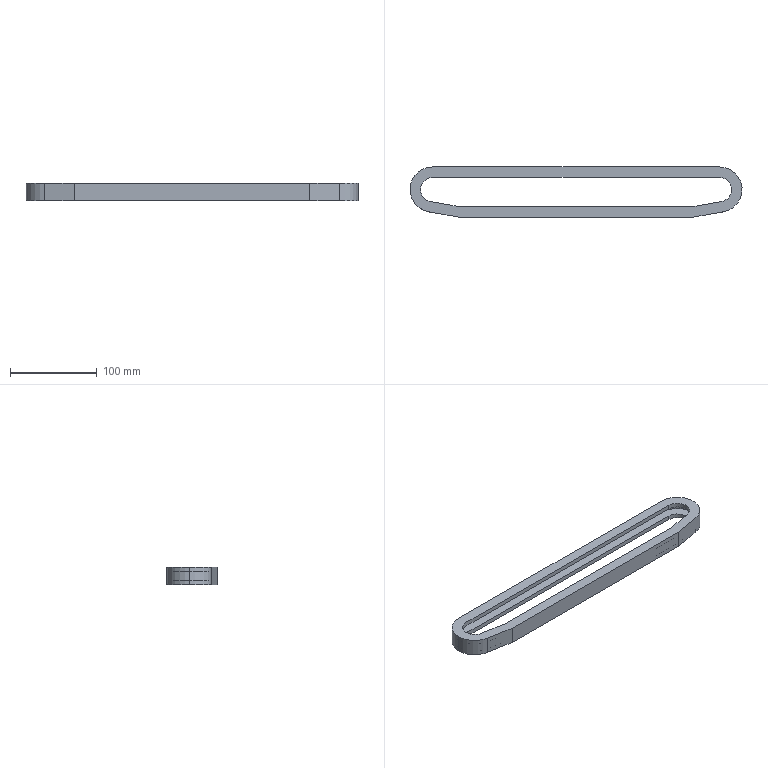Part | SolidWorks | features Extrusion 1, ICE 1 | 1 solid | 32 faces | box 382 x 57.598 x 20 mm | volume 102612 mm3 | plane 20 | cylinder 12 | commonest cylinder face diameters 28 x6 50 x3 52 x3
STEP:
#1=CARTESIAN_POINT('',(190.,0.,-5.));
#2=VERTEX_POINT('',#1);
#3=CARTESIAN_POINT('',(165.,25.,-5.));
#4=VERTEX_POINT('',#3);
#5=CARTESIAN_POINT('',(165.,0.,-5.));
#6=DIRECTION('',(0.,0.,1.));
#7=DIRECTION('',(1.,0.,0.));
#8=AXIS2_PLACEMENT_3D('',#5,#6,#7);
#9=CIRCLE('',#8,25.);
#10=EDGE_CURVE('',#2,#4,#9,.T.);
#11=ORIENTED_EDGE('',*,*,#10,.F.);
#12=CARTESIAN_POINT('',(190.,0.,5.));
#13=VERTEX_POINT('',#12);
#14=CARTESIAN_POINT('',(190.,0.,-5.));
#15=DIRECTION('',(0.,0.,1.));
#16=VECTOR('',#15,1000.);
#17=LINE('',#14,#16);
#18=EDGE_CURVE('',#2,#13,#17,.T.);
#19=ORIENTED_EDGE('',*,*,#18,.T.);
#20=CARTESIAN_POINT('',(165.,25.,5.));
#21=VERTEX_POINT('',#20);
#22=CARTESIAN_POINT('',(165.,0.,5.));
#23=DIRECTION('',(0.,0.,1.));
#24=DIRECTION('',(1.,0.,0.));
#25=AXIS2_PLACEMENT_3D('',#22,#23,#24);
#26=CIRCLE('',#25,25.);
#27=EDGE_CURVE('',#13,#21,#26,.T.);
#28=ORIENTED_EDGE('',*,*,#27,.T.);
#29=CARTESIAN_POINT('',(165.,25.,-5.));
#30=DIRECTION('',(0.,0.,1.));
#31=VECTOR('',#30,1000.);
#32=LINE('',#29,#31);
#33=EDGE_CURVE('',#4,#21,#32,.T.);
#34=ORIENTED_EDGE('',*,*,#33,.F.);
#35=EDGE_LOOP('',(#11,#19,#28,#34));
#36=FACE_OUTER_BOUND('',#35,.T.);
#37=CARTESIAN_POINT('',(165.,0.,-5.));
#38=DIRECTION('',(0.,0.,1.));
#39=DIRECTION('',(1.,0.,0.));
#40=AXIS2_PLACEMENT_3D('',#37,#38,#39);
#41=CYLINDRICAL_SURFACE('',#40,25.);
#42=ADVANCED_FACE('',(#36),#41,.F.);
#43=CARTESIAN_POINT('',(-165.,14.,10.));
#44=VERTEX_POINT('',#43);
#45=CARTESIAN_POINT('',(-179.,0.,10.));
#46=VERTEX_POINT('',#45);
#47=CARTESIAN_POINT('',(-165.,0.,10.));
#48=DIRECTION('',(0.,0.,1.));
#49=DIRECTION('',(1.,0.,0.));
#50=AXIS2_PLACEMENT_3D('',#47,#48,#49);
#51=CIRCLE('',#50,14.);
#52=EDGE_CURVE('',#44,#46,#51,.T.);
#53=ORIENTED_EDGE('',*,*,#52,.T.);
#54=CARTESIAN_POINT('',(-179.,0.,5.));
#55=VERTEX_POINT('',#54);
#56=CARTESIAN_POINT('',(-179.,0.,10.));
#57=DIRECTION('',(0.,0.,-1.));
#58=VECTOR('',#57,1000.);
#59=LINE('',#56,#58);
#60=EDGE_CURVE('',#46,#55,#59,.T.);
#61=ORIENTED_EDGE('',*,*,#60,.T.);
#62=CARTESIAN_POINT('',(-165.,14.,5.));
#63=VERTEX_POINT('',#62);
#64=CARTESIAN_POINT('',(-165.,0.,5.));
#65=DIRECTION('',(0.,0.,1.));
#66=DIRECTION('',(1.,0.,0.));
#67=AXIS2_PLACEMENT_3D('',#64,#65,#66);
#68=CIRCLE('',#67,14.);
#69=EDGE_CURVE('',#63,#55,#68,.T.);
#70=ORIENTED_EDGE('',*,*,#69,.F.);
#71=CARTESIAN_POINT('',(-165.,14.,10.));
#72=DIRECTION('',(0.,0.,-1.));
#73=VECTOR('',#72,1000.);
#74=LINE('',#71,#73);
#75=EDGE_CURVE('',#44,#63,#74,.T.);
#76=ORIENTED_EDGE('',*,*,#75,.F.);
#77=EDGE_LOOP('',(#53,#61,#70,#76));
#78=FACE_OUTER_BOUND('',#77,.T.);
#79=CARTESIAN_POINT('',(-165.,0.,10.));
#80=DIRECTION('',(0.,0.,-1.));
#81=DIRECTION('',(-1.,0.,0.));
#82=AXIS2_PLACEMENT_3D('',#79,#80,#81);
#83=CYLINDRICAL_SURFACE('',#82,14.);
#84=ADVANCED_FACE('',(#78),#83,.F.);
#85=CARTESIAN_POINT('',(-191.,0.,10.));
#86=VERTEX_POINT('',#85);
#87=CARTESIAN_POINT('',(-169.515,-25.605,10.));
#88=VERTEX_POINT('',#87);
#89=CARTESIAN_POINT('',(-165.,0.,10.));
#90=DIRECTION('',(0.,0.,1.));
#91=DIRECTION('',(1.,0.,0.));
#92=AXIS2_PLACEMENT_3D('',#89,#90,#91);
#93=CIRCLE('',#92,26.);
#94=EDGE_CURVE('',#86,#88,#93,.T.);
#95=ORIENTED_EDGE('',*,*,#94,.F.);
#96=CARTESIAN_POINT('',(-191.,0.,-10.));
#97=VERTEX_POINT('',#96);
#98=CARTESIAN_POINT('',(-191.,0.,10.));
#99=DIRECTION('',(0.,0.,-1.));
#100=VECTOR('',#99,1000.);
#101=LINE('',#98,#100);
#102=EDGE_CURVE('',#86,#97,#101,.T.);
#103=ORIENTED_EDGE('',*,*,#102,.T.);
#104=CARTESIAN_POINT('',(-169.515,-25.605,-10.));
#105=VERTEX_POINT('',#104);
#106=CARTESIAN_POINT('',(-165.,0.,-10.));
#107=DIRECTION('',(0.,0.,1.));
#108=DIRECTION('',(1.,0.,0.));
#109=AXIS2_PLACEMENT_3D('',#106,#107,#108);
#110=CIRCLE('',#109,26.);
#111=EDGE_CURVE('',#97,#105,#110,.T.);
#112=ORIENTED_EDGE('',*,*,#111,.T.);
#113=CARTESIAN_POINT('',(-169.515,-25.605,10.));
#114=DIRECTION('',(0.,0.,-1.));
#115=VECTOR('',#114,1000.);
#116=LINE('',#113,#115);
#117=EDGE_CURVE('',#88,#105,#116,.T.);
#118=ORIENTED_EDGE('',*,*,#117,.F.);
#119=EDGE_LOOP('',(#95,#103,#112,#118));
#120=FACE_OUTER_BOUND('',#119,.T.);
#121=CARTESIAN_POINT('',(-165.,0.,10.));
#122=DIRECTION('',(0.,0.,-1.));
#123=DIRECTION('',(-1.,0.,0.));
#124=AXIS2_PLACEMENT_3D('',#121,#122,#123);
#125=CYLINDRICAL_SURFACE('',#124,26.);
#126=ADVANCED_FACE('',(#120),#125,.T.);
#127=CARTESIAN_POINT('',(-165.,14.,-5.));
#128=VERTEX_POINT('',#127);
#129=CARTESIAN_POINT('',(-179.,0.,-5.));
#130=VERTEX_POINT('',#129);
#131=CARTESIAN_POINT('',(-165.,0.,-5.));
#132=DIRECTION('',(0.,0.,1.));
#133=DIRECTION('',(1.,0.,0.));
#134=AXIS2_PLACEMENT_3D('',#131,#132,#133);
#135=CIRCLE('',#134,14.);
#136=EDGE_CURVE('',#128,#130,#135,.T.);
#137=ORIENTED_EDGE('',*,*,#136,.T.);
#138=CARTESIAN_POINT('',(-179.,0.,-10.));
#139=VERTEX_POINT('',#138);
#140=CARTESIAN_POINT('',(-179.,0.,10.));
#141=DIRECTION('',(0.,0.,-1.));
#142=VECTOR('',#141,1000.);
#143=LINE('',#140,#142);
#144=EDGE_CURVE('',#130,#139,#143,.T.);
#145=ORIENTED_EDGE('',*,*,#144,.T.);
#146=CARTESIAN_POINT('',(-165.,14.,-10.));
#147=VERTEX_POINT('',#146);
#148=CARTESIAN_POINT('',(-165.,0.,-10.));
#149=DIRECTION('',(0.,0.,1.));
#150=DIRECTION('',(1.,0.,0.));
#151=AXIS2_PLACEMENT_3D('',#148,#149,#150);
#152=CIRCLE('',#151,14.);
#153=EDGE_CURVE('',#147,#139,#152,.T.);
#154=ORIENTED_EDGE('',*,*,#153,.F.);
#155=CARTESIAN_POINT('',(-165.,14.,10.));
#156=DIRECTION('',(0.,0.,-1.));
#157=VECTOR('',#156,1000.);
#158=LINE('',#155,#157);
#159=EDGE_CURVE('',#128,#147,#158,.T.);
#160=ORIENTED_EDGE('',*,*,#159,.F.);
#161=EDGE_LOOP('',(#137,#145,#154,#160));
#162=FACE_OUTER_BOUND('',#161,.T.);
#163=CARTESIAN_POINT('',(-165.,0.,10.));
#164=DIRECTION('',(0.,0.,-1.));
#165=DIRECTION('',(-1.,0.,0.));
#166=AXIS2_PLACEMENT_3D('',#163,#164,#165);
#167=CYLINDRICAL_SURFACE('',#166,14.);
#168=ADVANCED_FACE('',(#162),#167,.F.);
#169=ORIENTED_EDGE('',*,*,#144,.F.);
#170=CARTESIAN_POINT('',(-167.431,-13.787,-5.));
#171=VERTEX_POINT('',#170);
#172=CARTESIAN_POINT('',(-165.,0.,-5.));
#173=DIRECTION('',(0.,0.,1.));
#174=DIRECTION('',(1.,0.,0.));
#175=AXIS2_PLACEMENT_3D('',#172,#173,#174);
#176=CIRCLE('',#175,14.);
#177=EDGE_CURVE('',#130,#171,#176,.T.);
#178=ORIENTED_EDGE('',*,*,#177,.T.);
#179=CARTESIAN_POINT('',(-167.431,-13.787,-10.));
#180=VERTEX_POINT('',#179);
#181=CARTESIAN_POINT('',(-167.431,-13.787,10.));
#182=DIRECTION('',(0.,0.,-1.));
#183=VECTOR('',#182,1000.);
#184=LINE('',#181,#183);
#185=EDGE_CURVE('',#171,#180,#184,.T.);
#186=ORIENTED_EDGE('',*,*,#185,.T.);
#187=CARTESIAN_POINT('',(-165.,0.,-10.));
#188=DIRECTION('',(0.,0.,1.));
#189=DIRECTION('',(1.,0.,0.));
#190=AXIS2_PLACEMENT_3D('',#187,#188,#189);
#191=CIRCLE('',#190,14.);
#192=EDGE_CURVE('',#139,#180,#191,.T.);
#193=ORIENTED_EDGE('',*,*,#192,.F.);
#194=EDGE_LOOP('',(#169,#178,#186,#193));
#195=FACE_OUTER_BOUND('',#194,.T.);
#196=CARTESIAN_POINT('',(-165.,0.,10.));
#197=DIRECTION('',(0.,0.,-1.));
#198=DIRECTION('',(-1.,0.,0.));
#199=AXIS2_PLACEMENT_3D('',#196,#197,#198);
#200=CYLINDRICAL_SURFACE('',#199,14.);
#201=ADVANCED_FACE('',(#195),#200,.F.);
#202=ORIENTED_EDGE('',*,*,#185,.F.);
#203=CARTESIAN_POINT('',(-134.475,-19.598,-5.));
#204=VERTEX_POINT('',#203);
#205=CARTESIAN_POINT('',(-134.475,-19.598,-5.));
#206=DIRECTION('',(0.9848,-0.1736,0.));
#207=VECTOR('',#206,1000.);
#208=LINE('',#205,#207);
#209=EDGE_CURVE('',#171,#204,#208,.T.);
#210=ORIENTED_EDGE('',*,*,#209,.T.);
#211=CARTESIAN_POINT('',(-134.475,-19.598,-10.));
#212=VERTEX_POINT('',#211);
#213=CARTESIAN_POINT('',(-134.475,-19.598,10.));
#214=DIRECTION('',(0.,0.,-1.));
#215=VECTOR('',#214,1000.);
#216=LINE('',#213,#215);
#217=EDGE_CURVE('',#204,#212,#216,.T.);
#218=ORIENTED_EDGE('',*,*,#217,.T.);
#219=CARTESIAN_POINT('',(-134.475,-19.598,-10.));
#220=DIRECTION('',(0.9848,-0.1736,0.));
#221=VECTOR('',#220,1000.);
#222=LINE('',#219,#221);
#223=EDGE_CURVE('',#180,#212,#222,.T.);
#224=ORIENTED_EDGE('',*,*,#223,.F.);
#225=EDGE_LOOP('',(#202,#210,#218,#224));
#226=FACE_OUTER_BOUND('',#225,.T.);
#227=CARTESIAN_POINT('',(-134.475,-19.598,10.));
#228=DIRECTION('',(0.1736,0.9848,0.));
#229=DIRECTION('',(-0.9848,0.1736,0.));
#230=AXIS2_PLACEMENT_3D('',#227,#228,#229);
#231=PLANE('',#230);
#232=ADVANCED_FACE('',(#226),#231,.T.);
#233=ORIENTED_EDGE('',*,*,#217,.F.);
#234=CARTESIAN_POINT('',(134.475,-19.598,-5.));
#235=VERTEX_POINT('',#234);
#236=CARTESIAN_POINT('',(-134.475,-19.598,-5.));
#237=DIRECTION('',(1.,0.,0.));
#238=VECTOR('',#237,1000.);
#239=LINE('',#236,#238);
#240=EDGE_CURVE('',#204,#235,#239,.T.);
#241=ORIENTED_EDGE('',*,*,#240,.T.);
#242=CARTESIAN_POINT('',(134.475,-19.598,-10.));
#243=VERTEX_POINT('',#242);
#244=CARTESIAN_POINT('',(134.475,-19.598,10.));
#245=DIRECTION('',(0.,0.,-1.));
#246=VECTOR('',#245,1000.);
#247=LINE('',#244,#246);
#248=EDGE_CURVE('',#235,#243,#247,.T.);
#249=ORIENTED_EDGE('',*,*,#248,.T.);
#250=CARTESIAN_POINT('',(-134.475,-19.598,-10.));
#251=DIRECTION('',(1.,0.,0.));
#252=VECTOR('',#251,1000.);
#253=LINE('',#250,#252);
#254=EDGE_CURVE('',#212,#243,#253,.T.);
#255=ORIENTED_EDGE('',*,*,#254,.F.);
#256=EDGE_LOOP('',(#233,#241,#249,#255));
#257=FACE_OUTER_BOUND('',#256,.T.);
#258=CARTESIAN_POINT('',(-134.475,-19.598,10.));
#259=DIRECTION('',(0.,1.,0.));
#260=DIRECTION('',(0.,0.,1.));
#261=AXIS2_PLACEMENT_3D('',#258,#259,#260);
#262=PLANE('',#261);
#263=ADVANCED_FACE('',(#257),#262,.T.);
#264=ORIENTED_EDGE('',*,*,#248,.F.);
#265=CARTESIAN_POINT('',(167.431,-13.787,-5.));
#266=VERTEX_POINT('',#265);
#267=CARTESIAN_POINT('',(134.475,-19.598,-5.));
#268=DIRECTION('',(0.9848,0.1736,0.));
#269=VECTOR('',#268,1000.);
#270=LINE('',#267,#269);
#271=EDGE_CURVE('',#235,#266,#270,.T.);
#272=ORIENTED_EDGE('',*,*,#271,.T.);
#273=CARTESIAN_POINT('',(167.431,-13.787,-10.));
#274=VERTEX_POINT('',#273);
#275=CARTESIAN_POINT('',(167.431,-13.787,10.));
#276=DIRECTION('',(0.,0.,-1.));
#277=VECTOR('',#276,1000.);
#278=LINE('',#275,#277);
#279=EDGE_CURVE('',#266,#274,#278,.T.);
#280=ORIENTED_EDGE('',*,*,#279,.T.);
#281=CARTESIAN_POINT('',(134.475,-19.598,-10.));
#282=DIRECTION('',(0.9848,0.1736,0.));
#283=VECTOR('',#282,1000.);
#284=LINE('',#281,#283);
#285=EDGE_CURVE('',#243,#274,#284,.T.);
#286=ORIENTED_EDGE('',*,*,#285,.F.);
#287=EDGE_LOOP('',(#264,#272,#280,#286));
#288=FACE_OUTER_BOUND('',#287,.T.);
#289=CARTESIAN_POINT('',(134.475,-19.598,10.));
#290=DIRECTION('',(-0.1736,0.9848,0.));
#291=DIRECTION('',(-0.9848,-0.1736,0.));
#292=AXIS2_PLACEMENT_3D('',#289,#290,#291);
#293=PLANE('',#292);
#294=ADVANCED_FACE('',(#288),#293,.T.);
#295=ORIENTED_EDGE('',*,*,#279,.F.);
#296=CARTESIAN_POINT('',(165.,14.,-5.));
#297=VERTEX_POINT('',#296);
#298=CARTESIAN_POINT('',(165.,0.,-5.));
#299=DIRECTION('',(0.,0.,1.));
#300=DIRECTION('',(1.,0.,0.));
#301=AXIS2_PLACEMENT_3D('',#298,#299,#300);
#302=CIRCLE('',#301,14.);
#303=EDGE_CURVE('',#266,#297,#302,.T.);
#304=ORIENTED_EDGE('',*,*,#303,.T.);
#305=CARTESIAN_POINT('',(165.,14.,-10.));
#306=VERTEX_POINT('',#305);
#307=CARTESIAN_POINT('',(165.,14.,10.));
#308=DIRECTION('',(0.,0.,-1.));
#309=VECTOR('',#308,1000.);
#310=LINE('',#307,#309);
#311=EDGE_CURVE('',#297,#306,#310,.T.);
#312=ORIENTED_EDGE('',*,*,#311,.T.);
#313=CARTESIAN_POINT('',(165.,0.,-10.));
#314=DIRECTION('',(0.,0.,1.));
#315=DIRECTION('',(-1.,0.,0.));
#316=AXIS2_PLACEMENT_3D('',#313,#314,#315);
#317=CIRCLE('',#316,14.);
#318=EDGE_CURVE('',#274,#306,#317,.T.);
#319=ORIENTED_EDGE('',*,*,#318,.F.);
#320=EDGE_LOOP('',(#295,#304,#312,#319));
#321=FACE_OUTER_BOUND('',#320,.T.);
#322=CARTESIAN_POINT('',(165.,0.,10.));
#323=DIRECTION('',(0.,0.,-1.));
#324=DIRECTION('',(-1.,0.,0.));
#325=AXIS2_PLACEMENT_3D('',#322,#323,#324);
#326=CYLINDRICAL_SURFACE('',#325,14.);
#327=ADVANCED_FACE('',(#321),#326,.F.);
#328=ORIENTED_EDGE('',*,*,#311,.F.);
#329=CARTESIAN_POINT('',(-165.,14.,-5.));
#330=DIRECTION('',(-1.,0.,0.));
#331=VECTOR('',#330,1000.);
#332=LINE('',#329,#331);
#333=EDGE_CURVE('',#297,#128,#332,.T.);
#334=ORIENTED_EDGE('',*,*,#333,.T.);
#335=ORIENTED_EDGE('',*,*,#159,.T.);
#336=CARTESIAN_POINT('',(-165.,14.,-10.));
#337=DIRECTION('',(-1.,0.,0.));
#338=VECTOR('',#337,1000.);
#339=LINE('',#336,#338);
#340=EDGE_CURVE('',#306,#147,#339,.T.);
#341=ORIENTED_EDGE('',*,*,#340,.F.);
#342=EDGE_LOOP('',(#328,#334,#335,#341));
#343=FACE_OUTER_BOUND('',#342,.T.);
#344=CARTESIAN_POINT('',(-165.,14.,10.));
#345=DIRECTION('',(0.,-1.,0.));
#346=DIRECTION('',(0.,0.,-1.));
#347=AXIS2_PLACEMENT_3D('',#344,#345,#346);
#348=PLANE('',#347);
#349=ADVANCED_FACE('',(#343),#348,.T.);
#350=CARTESIAN_POINT('',(-165.,26.,10.));
#351=VERTEX_POINT('',#350);
#352=CARTESIAN_POINT('',(-165.,0.,10.));
#353=DIRECTION('',(0.,0.,1.));
#354=DIRECTION('',(1.,0.,0.));
#355=AXIS2_PLACEMENT_3D('',#352,#353,#354);
#356=CIRCLE('',#355,26.);
#357=EDGE_CURVE('',#351,#86,#356,.T.);
#358=ORIENTED_EDGE('',*,*,#357,.T.);
#359=ORIENTED_EDGE('',*,*,#94,.T.);
#360=CARTESIAN_POINT('',(-135.525,-31.598,10.));
#361=VERTEX_POINT('',#360);
#362=CARTESIAN_POINT('',(-135.525,-31.598,10.));
#363=DIRECTION('',(0.9848,-0.1736,0.));
#364=VECTOR('',#363,1000.);
#365=LINE('',#362,#364);
#366=EDGE_CURVE('',#88,#361,#365,.T.);
#367=ORIENTED_EDGE('',*,*,#366,.T.);
#368=CARTESIAN_POINT('',(135.525,-31.598,10.));
#369=VERTEX_POINT('',#368);
#370=CARTESIAN_POINT('',(-135.525,-31.598,10.));
#371=DIRECTION('',(1.,0.,0.));
#372=VECTOR('',#371,1000.);
#373=LINE('',#370,#372);
#374=EDGE_CURVE('',#361,#369,#373,.T.);
#375=ORIENTED_EDGE('',*,*,#374,.T.);
#376=CARTESIAN_POINT('',(169.515,-25.605,10.));
#377=VERTEX_POINT('',#376);
#378=CARTESIAN_POINT('',(135.525,-31.598,10.));
#379=DIRECTION('',(0.9848,0.1736,0.));
#380=VECTOR('',#379,1000.);
#381=LINE('',#378,#380);
#382=EDGE_CURVE('',#369,#377,#381,.T.);
#383=ORIENTED_EDGE('',*,*,#382,.T.);
#384=CARTESIAN_POINT('',(165.,26.,10.));
#385=VERTEX_POINT('',#384);
#386=CARTESIAN_POINT('',(165.,0.,10.));
#387=DIRECTION('',(0.,0.,1.));
#388=DIRECTION('',(-1.,0.,0.));
#389=AXIS2_PLACEMENT_3D('',#386,#387,#388);
#390=CIRCLE('',#389,26.);
#391=EDGE_CURVE('',#377,#385,#390,.T.);
#392=ORIENTED_EDGE('',*,*,#391,.T.);
#393=CARTESIAN_POINT('',(-165.,26.,10.));
#394=DIRECTION('',(-1.,0.,0.));
#395=VECTOR('',#394,1000.);
#396=LINE('',#393,#395);
#397=EDGE_CURVE('',#385,#351,#396,.T.);
#398=ORIENTED_EDGE('',*,*,#397,.T.);
#399=EDGE_LOOP('',(#358,#359,#367,#375,#383,#392,#398));
#400=FACE_OUTER_BOUND('',#399,.T.);
#401=CARTESIAN_POINT('',(-167.431,-13.787,10.));
#402=VERTEX_POINT('',#401);
#403=CARTESIAN_POINT('',(-134.475,-19.598,10.));
#404=VERTEX_POINT('',#403);
#405=CARTESIAN_POINT('',(-134.475,-19.598,10.));
#406=DIRECTION('',(0.9848,-0.1736,0.));
#407=VECTOR('',#406,1000.);
#408=LINE('',#405,#407);
#409=EDGE_CURVE('',#402,#404,#408,.T.);
#410=ORIENTED_EDGE('',*,*,#409,.F.);
#411=CARTESIAN_POINT('',(-165.,0.,10.));
#412=DIRECTION('',(0.,0.,1.));
#413=DIRECTION('',(1.,0.,0.));
#414=AXIS2_PLACEMENT_3D('',#411,#412,#413);
#415=CIRCLE('',#414,14.);
#416=EDGE_CURVE('',#46,#402,#415,.T.);
#417=ORIENTED_EDGE('',*,*,#416,.F.);
#418=ORIENTED_EDGE('',*,*,#52,.F.);
#419=CARTESIAN_POINT('',(165.,14.,10.));
#420=VERTEX_POINT('',#419);
#421=CARTESIAN_POINT('',(-165.,14.,10.));
#422=DIRECTION('',(-1.,0.,0.));
#423=VECTOR('',#422,1000.);
#424=LINE('',#421,#423);
#425=EDGE_CURVE('',#420,#44,#424,.T.);
#426=ORIENTED_EDGE('',*,*,#425,.F.);
#427=CARTESIAN_POINT('',(167.431,-13.787,10.));
#428=VERTEX_POINT('',#427);
#429=CARTESIAN_POINT('',(165.,0.,10.));
#430=DIRECTION('',(0.,0.,1.));
#431=DIRECTION('',(-1.,0.,0.));
#432=AXIS2_PLACEMENT_3D('',#429,#430,#431);
#433=CIRCLE('',#432,14.);
#434=EDGE_CURVE('',#428,#420,#433,.T.);
#435=ORIENTED_EDGE('',*,*,#434,.F.);
#436=CARTESIAN_POINT('',(134.475,-19.598,10.));
#437=VERTEX_POINT('',#436);
#438=CARTESIAN_POINT('',(134.475,-19.598,10.));
#439=DIRECTION('',(0.9848,0.1736,0.));
#440=VECTOR('',#439,1000.);
#441=LINE('',#438,#440);
#442=EDGE_CURVE('',#437,#428,#441,.T.);
#443=ORIENTED_EDGE('',*,*,#442,.F.);
#444=CARTESIAN_POINT('',(-134.475,-19.598,10.));
#445=DIRECTION('',(1.,0.,0.));
#446=VECTOR('',#445,1000.);
#447=LINE('',#444,#446);
#448=EDGE_CURVE('',#404,#437,#447,.T.);
#449=ORIENTED_EDGE('',*,*,#448,.F.);
#450=EDGE_LOOP('',(#410,#417,#418,#426,#435,#443,#449));
#451=FACE_BOUND('',#450,.T.);
#452=CARTESIAN_POINT('',(-165.,0.,10.));
#453=DIRECTION('',(0.,0.,1.));
#454=DIRECTION('',(1.,0.,0.));
#455=AXIS2_PLACEMENT_3D('',#452,#453,#454);
#456=PLANE('',#455);
#457=ADVANCED_FACE('',(#400,#451),#456,.T.);
#458=CARTESIAN_POINT('',(-165.,26.,-10.));
#459=VERTEX_POINT('',#458);
#460=CARTESIAN_POINT('',(-165.,0.,-10.));
#461=DIRECTION('',(0.,0.,1.));
#462=DIRECTION('',(1.,0.,0.));
#463=AXIS2_PLACEMENT_3D('',#460,#461,#462);
#464=CIRCLE('',#463,26.);
#465=EDGE_CURVE('',#459,#97,#464,.T.);
#466=ORIENTED_EDGE('',*,*,#465,.F.);
#467=CARTESIAN_POINT('',(165.,26.,-10.));
#468=VERTEX_POINT('',#467);
#469=CARTESIAN_POINT('',(-165.,26.,-10.));
#470=DIRECTION('',(-1.,0.,0.));
#471=VECTOR('',#470,1000.);
#472=LINE('',#469,#471);
#473=EDGE_CURVE('',#468,#459,#472,.T.);
#474=ORIENTED_EDGE('',*,*,#473,.F.);
#475=CARTESIAN_POINT('',(169.515,-25.605,-10.));
#476=VERTEX_POINT('',#475);
#477=CARTESIAN_POINT('',(165.,0.,-10.));
#478=DIRECTION('',(0.,0.,1.));
#479=DIRECTION('',(-1.,0.,0.));
#480=AXIS2_PLACEMENT_3D('',#477,#478,#479);
#481=CIRCLE('',#480,26.);
#482=EDGE_CURVE('',#476,#468,#481,.T.);
#483=ORIENTED_EDGE('',*,*,#482,.F.);
#484=CARTESIAN_POINT('',(135.525,-31.598,-10.));
#485=VERTEX_POINT('',#484);
#486=CARTESIAN_POINT('',(135.525,-31.598,-10.));
#487=DIRECTION('',(0.9848,0.1736,0.));
#488=VECTOR('',#487,1000.);
#489=LINE('',#486,#488);
#490=EDGE_CURVE('',#485,#476,#489,.T.);
#491=ORIENTED_EDGE('',*,*,#490,.F.);
#492=CARTESIAN_POINT('',(-135.525,-31.598,-10.));
#493=VERTEX_POINT('',#492);
#494=CARTESIAN_POINT('',(-135.525,-31.598,-10.));
#495=DIRECTION('',(1.,0.,0.));
#496=VECTOR('',#495,1000.);
#497=LINE('',#494,#496);
#498=EDGE_CURVE('',#493,#485,#497,.T.);
#499=ORIENTED_EDGE('',*,*,#498,.F.);
#500=CARTESIAN_POINT('',(-135.525,-31.598,-10.));
#501=DIRECTION('',(0.9848,-0.1736,0.));
#502=VECTOR('',#501,1000.);
#503=LINE('',#500,#502);
#504=EDGE_CURVE('',#105,#493,#503,.T.);
#505=ORIENTED_EDGE('',*,*,#504,.F.);
#506=ORIENTED_EDGE('',*,*,#111,.F.);
#507=EDGE_LOOP('',(#466,#474,#483,#491,#499,#505,#506));
#508=FACE_OUTER_BOUND('',#507,.T.);
#509=ORIENTED_EDGE('',*,*,#153,.T.);
#510=ORIENTED_EDGE('',*,*,#192,.T.);
#511=ORIENTED_EDGE('',*,*,#223,.T.);
#512=ORIENTED_EDGE('',*,*,#254,.T.);
#513=ORIENTED_EDGE('',*,*,#285,.T.);
#514=ORIENTED_EDGE('',*,*,#318,.T.);
#515=ORIENTED_EDGE('',*,*,#340,.T.);
#516=EDGE_LOOP('',(#509,#510,#511,#512,#513,#514,#515));
#517=FACE_BOUND('',#516,.T.);
#518=CARTESIAN_POINT('',(-165.,0.,-10.));
#519=DIRECTION('',(0.,0.,1.));
#520=DIRECTION('',(1.,0.,0.));
#521=AXIS2_PLACEMENT_3D('',#518,#519,#520);
#522=PLANE('',#521);
#523=ADVANCED_FACE('',(#508,#517),#522,.F.);
#524=ORIENTED_EDGE('',*,*,#102,.F.);
#525=ORIENTED_EDGE('',*,*,#357,.F.);
#526=CARTESIAN_POINT('',(-165.,26.,10.));
#527=DIRECTION('',(0.,0.,-1.));
#528=VECTOR('',#527,1000.);
#529=LINE('',#526,#528);
#530=EDGE_CURVE('',#351,#459,#529,.T.);
#531=ORIENTED_EDGE('',*,*,#530,.T.);
#532=ORIENTED_EDGE('',*,*,#465,.T.);
#533=EDGE_LOOP('',(#524,#525,#531,#532));
#534=FACE_OUTER_BOUND('',#533,.T.);
#535=CARTESIAN_POINT('',(-165.,0.,10.));
#536=DIRECTION('',(0.,0.,-1.));
#537=DIRECTION('',(-1.,0.,0.));
#538=AXIS2_PLACEMENT_3D('',#535,#536,#537);
#539=CYLINDRICAL_SURFACE('',#538,26.);
#540=ADVANCED_FACE('',(#534),#539,.T.);
#541=ORIENTED_EDGE('',*,*,#504,.T.);
#542=CARTESIAN_POINT('',(-135.525,-31.598,10.));
#543=DIRECTION('',(0.,0.,-1.));
#544=VECTOR('',#543,1000.);
#545=LINE('',#542,#544);
#546=EDGE_CURVE('',#361,#493,#545,.T.);
#547=ORIENTED_EDGE('',*,*,#546,.F.);
#548=ORIENTED_EDGE('',*,*,#366,.F.);
#549=ORIENTED_EDGE('',*,*,#117,.T.);
#550=EDGE_LOOP('',(#541,#547,#548,#549));
#551=FACE_OUTER_BOUND('',#550,.T.);
#552=CARTESIAN_POINT('',(-135.525,-31.598,10.));
#553=DIRECTION('',(0.1736,0.9848,0.));
#554=DIRECTION('',(-0.9848,0.1736,0.));
#555=AXIS2_PLACEMENT_3D('',#552,#553,#554);
#556=PLANE('',#555);
#557=ADVANCED_FACE('',(#551),#556,.F.);
#558=ORIENTED_EDGE('',*,*,#498,.T.);
#559=CARTESIAN_POINT('',(135.525,-31.598,10.));
#560=DIRECTION('',(0.,0.,-1.));
#561=VECTOR('',#560,1000.);
#562=LINE('',#559,#561);
#563=EDGE_CURVE('',#369,#485,#562,.T.);
#564=ORIENTED_EDGE('',*,*,#563,.F.);
#565=ORIENTED_EDGE('',*,*,#374,.F.);
#566=ORIENTED_EDGE('',*,*,#546,.T.);
#567=EDGE_LOOP('',(#558,#564,#565,#566));
#568=FACE_OUTER_BOUND('',#567,.T.);
#569=CARTESIAN_POINT('',(-135.525,-31.598,10.));
#570=DIRECTION('',(0.,1.,0.));
#571=DIRECTION('',(0.,0.,1.));
#572=AXIS2_PLACEMENT_3D('',#569,#570,#571);
#573=PLANE('',#572);
#574=ADVANCED_FACE('',(#568),#573,.F.);
#575=ORIENTED_EDGE('',*,*,#490,.T.);
#576=CARTESIAN_POINT('',(169.515,-25.605,10.));
#577=DIRECTION('',(0.,0.,-1.));
#578=VECTOR('',#577,1000.);
#579=LINE('',#576,#578);
#580=EDGE_CURVE('',#377,#476,#579,.T.);
#581=ORIENTED_EDGE('',*,*,#580,.F.);
#582=ORIENTED_EDGE('',*,*,#382,.F.);
#583=ORIENTED_EDGE('',*,*,#563,.T.);
#584=EDGE_LOOP('',(#575,#581,#582,#583));
#585=FACE_OUTER_BOUND('',#584,.T.);
#586=CARTESIAN_POINT('',(135.525,-31.598,10.));
#587=DIRECTION('',(-0.1736,0.9848,0.));
#588=DIRECTION('',(-0.9848,-0.1736,0.));
#589=AXIS2_PLACEMENT_3D('',#586,#587,#588);
#590=PLANE('',#589);
#591=ADVANCED_FACE('',(#585),#590,.F.);
#592=ORIENTED_EDGE('',*,*,#482,.T.);
#593=CARTESIAN_POINT('',(165.,26.,10.));
#594=DIRECTION('',(0.,0.,-1.));
#595=VECTOR('',#594,1000.);
#596=LINE('',#593,#595);
#597=EDGE_CURVE('',#385,#468,#596,.T.);
#598=ORIENTED_EDGE('',*,*,#597,.F.);
#599=ORIENTED_EDGE('',*,*,#391,.F.);
#600=ORIENTED_EDGE('',*,*,#580,.T.);
#601=EDGE_LOOP('',(#592,#598,#599,#600));
#602=FACE_OUTER_BOUND('',#601,.T.);
#603=CARTESIAN_POINT('',(165.,0.,10.));
#604=DIRECTION('',(0.,0.,-1.));
#605=DIRECTION('',(-1.,0.,0.));
#606=AXIS2_PLACEMENT_3D('',#603,#604,#605);
#607=CYLINDRICAL_SURFACE('',#606,26.);
#608=ADVANCED_FACE('',(#602),#607,.T.);
#609=ORIENTED_EDGE('',*,*,#473,.T.);
#610=ORIENTED_EDGE('',*,*,#530,.F.);
#611=ORIENTED_EDGE('',*,*,#397,.F.);
#612=ORIENTED_EDGE('',*,*,#597,.T.);
#613=EDGE_LOOP('',(#609,#610,#611,#612));
#614=FACE_OUTER_BOUND('',#613,.T.);
#615=CARTESIAN_POINT('',(-165.,26.,10.));
#616=DIRECTION('',(0.,-1.,0.));
#617=DIRECTION('',(0.,0.,-1.));
#618=AXIS2_PLACEMENT_3D('',#615,#616,#617);
#619=PLANE('',#618);
#620=ADVANCED_FACE('',(#614),#619,.F.);
#621=ORIENTED_EDGE('',*,*,#60,.F.);
#622=ORIENTED_EDGE('',*,*,#416,.T.);
#623=CARTESIAN_POINT('',(-167.431,-13.787,5.));
#624=VERTEX_POINT('',#623);
#625=CARTESIAN_POINT('',(-167.431,-13.787,10.));
#626=DIRECTION('',(0.,0.,-1.));
#627=VECTOR('',#626,1000.);
#628=LINE('',#625,#627);
#629=EDGE_CURVE('',#402,#624,#628,.T.);
#630=ORIENTED_EDGE('',*,*,#629,.T.);
#631=CARTESIAN_POINT('',(-165.,0.,5.));
#632=DIRECTION('',(0.,0.,1.));
#633=DIRECTION('',(1.,0.,0.));
#634=AXIS2_PLACEMENT_3D('',#631,#632,#633);
#635=CIRCLE('',#634,14.);
#636=EDGE_CURVE('',#55,#624,#635,.T.);
#637=ORIENTED_EDGE('',*,*,#636,.F.);
#638=EDGE_LOOP('',(#621,#622,#630,#637));
#639=FACE_OUTER_BOUND('',#638,.T.);
#640=CARTESIAN_POINT('',(-165.,0.,10.));
#641=DIRECTION('',(0.,0.,-1.));
#642=DIRECTION('',(-1.,0.,0.));
#643=AXIS2_PLACEMENT_3D('',#640,#641,#642);
#644=CYLINDRICAL_SURFACE('',#643,14.);
#645=ADVANCED_FACE('',(#639),#644,.F.);
#646=CARTESIAN_POINT('',(-134.475,-19.598,5.));
#647=VERTEX_POINT('',#646);
#648=CARTESIAN_POINT('',(-134.475,-19.598,5.));
#649=DIRECTION('',(0.9848,-0.1736,0.));
#650=VECTOR('',#649,1000.);
#651=LINE('',#648,#650);
#652=EDGE_CURVE('',#624,#647,#651,.T.);
#653=ORIENTED_EDGE('',*,*,#652,.F.);
#654=ORIENTED_EDGE('',*,*,#629,.F.);
#655=ORIENTED_EDGE('',*,*,#409,.T.);
#656=CARTESIAN_POINT('',(-134.475,-19.598,10.));
#657=DIRECTION('',(0.,0.,-1.));
#658=VECTOR('',#657,1000.);
#659=LINE('',#656,#658);
#660=EDGE_CURVE('',#404,#647,#659,.T.);
#661=ORIENTED_EDGE('',*,*,#660,.T.);
#662=EDGE_LOOP('',(#653,#654,#655,#661));
#663=FACE_OUTER_BOUND('',#662,.T.);
#664=CARTESIAN_POINT('',(-134.475,-19.598,10.));
#665=DIRECTION('',(0.1736,0.9848,0.));
#666=DIRECTION('',(-0.9848,0.1736,0.));
#667=AXIS2_PLACEMENT_3D('',#664,#665,#666);
#668=PLANE('',#667);
#669=ADVANCED_FACE('',(#663),#668,.T.);
#670=CARTESIAN_POINT('',(134.475,-19.598,5.));
#671=VERTEX_POINT('',#670);
#672=CARTESIAN_POINT('',(-134.475,-19.598,5.));
#673=DIRECTION('',(1.,0.,0.));
#674=VECTOR('',#673,1000.);
#675=LINE('',#672,#674);
#676=EDGE_CURVE('',#647,#671,#675,.T.);
#677=ORIENTED_EDGE('',*,*,#676,.F.);
#678=ORIENTED_EDGE('',*,*,#660,.F.);
#679=ORIENTED_EDGE('',*,*,#448,.T.);
#680=CARTESIAN_POINT('',(134.475,-19.598,10.));
#681=DIRECTION('',(0.,0.,-1.));
#682=VECTOR('',#681,1000.);
#683=LINE('',#680,#682);
#684=EDGE_CURVE('',#437,#671,#683,.T.);
#685=ORIENTED_EDGE('',*,*,#684,.T.);
#686=EDGE_LOOP('',(#677,#678,#679,#685));
#687=FACE_OUTER_BOUND('',#686,.T.);
#688=CARTESIAN_POINT('',(-134.475,-19.598,10.));
#689=DIRECTION('',(0.,1.,0.));
#690=DIRECTION('',(0.,0.,1.));
#691=AXIS2_PLACEMENT_3D('',#688,#689,#690);
#692=PLANE('',#691);
#693=ADVANCED_FACE('',(#687),#692,.T.);
#694=CARTESIAN_POINT('',(167.431,-13.787,5.));
#695=VERTEX_POINT('',#694);
#696=CARTESIAN_POINT('',(134.475,-19.598,5.));
#697=DIRECTION('',(0.9848,0.1736,0.));
#698=VECTOR('',#697,1000.);
#699=LINE('',#696,#698);
#700=EDGE_CURVE('',#671,#695,#699,.T.);
#701=ORIENTED_EDGE('',*,*,#700,.F.);
#702=ORIENTED_EDGE('',*,*,#684,.F.);
#703=ORIENTED_EDGE('',*,*,#442,.T.);
#704=CARTESIAN_POINT('',(167.431,-13.787,10.));
#705=DIRECTION('',(0.,0.,-1.));
#706=VECTOR('',#705,1000.);
#707=LINE('',#704,#706);
#708=EDGE_CURVE('',#428,#695,#707,.T.);
#709=ORIENTED_EDGE('',*,*,#708,.T.);
#710=EDGE_LOOP('',(#701,#702,#703,#709));
#711=FACE_OUTER_BOUND('',#710,.T.);
#712=CARTESIAN_POINT('',(134.475,-19.598,10.));
#713=DIRECTION('',(-0.1736,0.9848,0.));
#714=DIRECTION('',(-0.9848,-0.1736,0.));
#715=AXIS2_PLACEMENT_3D('',#712,#713,#714);
#716=PLANE('',#715);
#717=ADVANCED_FACE('',(#711),#716,.T.);
#718=CARTESIAN_POINT('',(165.,14.,5.));
#719=VERTEX_POINT('',#718);
#720=CARTESIAN_POINT('',(165.,0.,5.));
#721=DIRECTION('',(0.,0.,1.));
#722=DIRECTION('',(1.,0.,0.));
#723=AXIS2_PLACEMENT_3D('',#720,#721,#722);
#724=CIRCLE('',#723,14.);
#725=EDGE_CURVE('',#695,#719,#724,.T.);
#726=ORIENTED_EDGE('',*,*,#725,.F.);
#727=ORIENTED_EDGE('',*,*,#708,.F.);
#728=ORIENTED_EDGE('',*,*,#434,.T.);
#729=CARTESIAN_POINT('',(165.,14.,10.));
#730=DIRECTION('',(0.,0.,-1.));
#731=VECTOR('',#730,1000.);
#732=LINE('',#729,#731);
#733=EDGE_CURVE('',#420,#719,#732,.T.);
#734=ORIENTED_EDGE('',*,*,#733,.T.);
#735=EDGE_LOOP('',(#726,#727,#728,#734));
#736=FACE_OUTER_BOUND('',#735,.T.);
#737=CARTESIAN_POINT('',(165.,0.,10.));
#738=DIRECTION('',(0.,0.,-1.));
#739=DIRECTION('',(-1.,0.,0.));
#740=AXIS2_PLACEMENT_3D('',#737,#738,#739);
#741=CYLINDRICAL_SURFACE('',#740,14.);
#742=ADVANCED_FACE('',(#736),#741,.F.);
#743=CARTESIAN_POINT('',(-165.,14.,5.));
#744=DIRECTION('',(-1.,0.,0.));
#745=VECTOR('',#744,1000.);
#746=LINE('',#743,#745);
#747=EDGE_CURVE('',#719,#63,#746,.T.);
#748=ORIENTED_EDGE('',*,*,#747,.F.);
#749=ORIENTED_EDGE('',*,*,#733,.F.);
#750=ORIENTED_EDGE('',*,*,#425,.T.);
#751=ORIENTED_EDGE('',*,*,#75,.T.);
#752=EDGE_LOOP('',(#748,#749,#750,#751));
#753=FACE_OUTER_BOUND('',#752,.T.);
#754=CARTESIAN_POINT('',(-165.,14.,10.));
#755=DIRECTION('',(0.,-1.,0.));
#756=DIRECTION('',(0.,0.,-1.));
#757=AXIS2_PLACEMENT_3D('',#754,#755,#756);
#758=PLANE('',#757);
#759=ADVANCED_FACE('',(#753),#758,.T.);
#760=CARTESIAN_POINT('',(-135.437,-30.598,5.));
#761=VERTEX_POINT('',#760);
#762=CARTESIAN_POINT('',(135.437,-30.598,5.));
#763=VERTEX_POINT('',#762);
#764=CARTESIAN_POINT('',(-135.437,-30.598,5.));
#765=DIRECTION('',(1.,0.,0.));
#766=VECTOR('',#765,1000.);
#767=LINE('',#764,#766);
#768=EDGE_CURVE('',#761,#763,#767,.T.);
#769=ORIENTED_EDGE('',*,*,#768,.T.);
#770=CARTESIAN_POINT('',(135.437,-30.598,-5.));
#771=VERTEX_POINT('',#770);
#772=CARTESIAN_POINT('',(135.437,-30.598,-5.));
#773=DIRECTION('',(0.,0.,1.));
#774=VECTOR('',#773,1000.);
#775=LINE('',#772,#774);
#776=EDGE_CURVE('',#771,#763,#775,.T.);
#777=ORIENTED_EDGE('',*,*,#776,.F.);
#778=CARTESIAN_POINT('',(-135.437,-30.598,-5.));
#779=VERTEX_POINT('',#778);
#780=CARTESIAN_POINT('',(-135.437,-30.598,-5.));
#781=DIRECTION('',(1.,0.,0.));
#782=VECTOR('',#781,1000.);
#783=LINE('',#780,#782);
#784=EDGE_CURVE('',#779,#771,#783,.T.);
#785=ORIENTED_EDGE('',*,*,#784,.F.);
#786=CARTESIAN_POINT('',(-135.437,-30.598,-5.));
#787=DIRECTION('',(0.,0.,1.));
#788=VECTOR('',#787,1000.);
#789=LINE('',#786,#788);
#790=EDGE_CURVE('',#779,#761,#789,.T.);
#791=ORIENTED_EDGE('',*,*,#790,.T.);
#792=EDGE_LOOP('',(#769,#777,#785,#791));
#793=FACE_OUTER_BOUND('',#792,.T.);
#794=CARTESIAN_POINT('',(-135.437,-30.598,-5.));
#795=DIRECTION('',(0.,-1.,0.));
#796=DIRECTION('',(0.,0.,-1.));
#797=AXIS2_PLACEMENT_3D('',#794,#795,#796);
#798=PLANE('',#797);
#799=ADVANCED_FACE('',(#793),#798,.F.);
#800=CARTESIAN_POINT('',(-169.341,-24.62,5.));
#801=VERTEX_POINT('',#800);
#802=CARTESIAN_POINT('',(-169.341,-24.62,5.));
#803=DIRECTION('',(0.9848,-0.1736,0.));
#804=VECTOR('',#803,1000.);
#805=LINE('',#802,#804);
#806=EDGE_CURVE('',#801,#761,#805,.T.);
#807=ORIENTED_EDGE('',*,*,#806,.T.);
#808=ORIENTED_EDGE('',*,*,#790,.F.);
#809=CARTESIAN_POINT('',(-169.341,-24.62,-5.));
#810=VERTEX_POINT('',#809);
#811=CARTESIAN_POINT('',(-169.341,-24.62,-5.));
#812=DIRECTION('',(0.9848,-0.1736,0.));
#813=VECTOR('',#812,1000.);
#814=LINE('',#811,#813);
#815=EDGE_CURVE('',#810,#779,#814,.T.);
#816=ORIENTED_EDGE('',*,*,#815,.F.);
#817=CARTESIAN_POINT('',(-169.341,-24.62,-5.));
#818=DIRECTION('',(0.,0.,1.));
#819=VECTOR('',#818,1000.);
#820=LINE('',#817,#819);
#821=EDGE_CURVE('',#810,#801,#820,.T.);
#822=ORIENTED_EDGE('',*,*,#821,.T.);
#823=EDGE_LOOP('',(#807,#808,#816,#822));
#824=FACE_OUTER_BOUND('',#823,.T.);
#825=CARTESIAN_POINT('',(-169.341,-24.62,-5.));
#826=DIRECTION('',(-0.1736,-0.9848,0.));
#827=DIRECTION('',(0.9848,-0.1736,0.));
#828=AXIS2_PLACEMENT_3D('',#825,#826,#827);
#829=PLANE('',#828);
#830=ADVANCED_FACE('',(#824),#829,.F.);
#831=CARTESIAN_POINT('',(-165.,25.,5.));
#832=VERTEX_POINT('',#831);
#833=CARTESIAN_POINT('',(-165.,0.,5.));
#834=DIRECTION('',(0.,0.,1.));
#835=DIRECTION('',(1.,0.,0.));
#836=AXIS2_PLACEMENT_3D('',#833,#834,#835);
#837=CIRCLE('',#836,25.);
#838=EDGE_CURVE('',#832,#801,#837,.T.);
#839=ORIENTED_EDGE('',*,*,#838,.T.);
#840=ORIENTED_EDGE('',*,*,#821,.F.);
#841=CARTESIAN_POINT('',(-165.,25.,-5.));
#842=VERTEX_POINT('',#841);
#843=CARTESIAN_POINT('',(-165.,0.,-5.));
#844=DIRECTION('',(0.,0.,1.));
#845=DIRECTION('',(1.,0.,0.));
#846=AXIS2_PLACEMENT_3D('',#843,#844,#845);
#847=CIRCLE('',#846,25.);
#848=EDGE_CURVE('',#842,#810,#847,.T.);
#849=ORIENTED_EDGE('',*,*,#848,.F.);
#850=CARTESIAN_POINT('',(-165.,25.,-5.));
#851=DIRECTION('',(0.,0.,1.));
#852=VECTOR('',#851,1000.);
#853=LINE('',#850,#852);
#854=EDGE_CURVE('',#842,#832,#853,.T.);
#855=ORIENTED_EDGE('',*,*,#854,.T.);
#856=EDGE_LOOP('',(#839,#840,#849,#855));
#857=FACE_OUTER_BOUND('',#856,.T.);
#858=CARTESIAN_POINT('',(-165.,0.,-5.));
#859=DIRECTION('',(0.,0.,1.));
#860=DIRECTION('',(1.,0.,0.));
#861=AXIS2_PLACEMENT_3D('',#858,#859,#860);
#862=CYLINDRICAL_SURFACE('',#861,25.);
#863=ADVANCED_FACE('',(#857),#862,.F.);
#864=CARTESIAN_POINT('',(165.,25.,5.));
#865=DIRECTION('',(-1.,0.,0.));
#866=VECTOR('',#865,1000.);
#867=LINE('',#864,#866);
#868=EDGE_CURVE('',#21,#832,#867,.T.);
#869=ORIENTED_EDGE('',*,*,#868,.T.);
#870=ORIENTED_EDGE('',*,*,#854,.F.);
#871=CARTESIAN_POINT('',(165.,25.,-5.));
#872=DIRECTION('',(-1.,0.,0.));
#873=VECTOR('',#872,1000.);
#874=LINE('',#871,#873);
#875=EDGE_CURVE('',#4,#842,#874,.T.);
#876=ORIENTED_EDGE('',*,*,#875,.F.);
#877=ORIENTED_EDGE('',*,*,#33,.T.);
#878=EDGE_LOOP('',(#869,#870,#876,#877));
#879=FACE_OUTER_BOUND('',#878,.T.);
#880=CARTESIAN_POINT('',(165.,25.,-5.));
#881=DIRECTION('',(0.,1.,0.));
#882=DIRECTION('',(0.,0.,1.));
#883=AXIS2_PLACEMENT_3D('',#880,#881,#882);
#884=PLANE('',#883);
#885=ADVANCED_FACE('',(#879),#884,.F.);
#886=ORIENTED_EDGE('',*,*,#18,.F.);
#887=CARTESIAN_POINT('',(169.341,-24.62,-5.));
#888=VERTEX_POINT('',#887);
#889=CARTESIAN_POINT('',(165.,0.,-5.));
#890=DIRECTION('',(0.,0.,1.));
#891=DIRECTION('',(1.,0.,0.));
#892=AXIS2_PLACEMENT_3D('',#889,#890,#891);
#893=CIRCLE('',#892,25.);
#894=EDGE_CURVE('',#888,#2,#893,.T.);
#895=ORIENTED_EDGE('',*,*,#894,.F.);
#896=CARTESIAN_POINT('',(169.341,-24.62,5.));
#897=VERTEX_POINT('',#896);
#898=CARTESIAN_POINT('',(169.341,-24.62,-5.));
#899=DIRECTION('',(0.,0.,1.));
#900=VECTOR('',#899,1000.);
#901=LINE('',#898,#900);
#902=EDGE_CURVE('',#888,#897,#901,.T.);
#903=ORIENTED_EDGE('',*,*,#902,.T.);
#904=CARTESIAN_POINT('',(165.,0.,5.));
#905=DIRECTION('',(0.,0.,1.));
#906=DIRECTION('',(1.,0.,0.));
#907=AXIS2_PLACEMENT_3D('',#904,#905,#906);
#908=CIRCLE('',#907,25.);
#909=EDGE_CURVE('',#897,#13,#908,.T.);
#910=ORIENTED_EDGE('',*,*,#909,.T.);
#911=EDGE_LOOP('',(#886,#895,#903,#910));
#912=FACE_OUTER_BOUND('',#911,.T.);
#913=CARTESIAN_POINT('',(165.,0.,-5.));
#914=DIRECTION('',(0.,0.,1.));
#915=DIRECTION('',(1.,0.,0.));
#916=AXIS2_PLACEMENT_3D('',#913,#914,#915);
#917=CYLINDRICAL_SURFACE('',#916,25.);
#918=ADVANCED_FACE('',(#912),#917,.F.);
#919=CARTESIAN_POINT('',(135.437,-30.598,5.));
#920=DIRECTION('',(0.9848,0.1736,0.));
#921=VECTOR('',#920,1000.);
#922=LINE('',#919,#921);
#923=EDGE_CURVE('',#763,#897,#922,.T.);
#924=ORIENTED_EDGE('',*,*,#923,.T.);
#925=ORIENTED_EDGE('',*,*,#902,.F.);
#926=CARTESIAN_POINT('',(135.437,-30.598,-5.));
#927=DIRECTION('',(0.9848,0.1736,0.));
#928=VECTOR('',#927,1000.);
#929=LINE('',#926,#928);
#930=EDGE_CURVE('',#771,#888,#929,.T.);
#931=ORIENTED_EDGE('',*,*,#930,.F.);
#932=ORIENTED_EDGE('',*,*,#776,.T.);
#933=EDGE_LOOP('',(#924,#925,#931,#932));
#934=FACE_OUTER_BOUND('',#933,.T.);
#935=CARTESIAN_POINT('',(135.437,-30.598,-5.));
#936=DIRECTION('',(0.1736,-0.9848,0.));
#937=DIRECTION('',(0.9848,0.1736,0.));
#938=AXIS2_PLACEMENT_3D('',#935,#936,#937);
#939=PLANE('',#938);
#940=ADVANCED_FACE('',(#934),#939,.F.);
#941=ORIENTED_EDGE('',*,*,#333,.F.);
#942=ORIENTED_EDGE('',*,*,#303,.F.);
#943=ORIENTED_EDGE('',*,*,#271,.F.);
#944=ORIENTED_EDGE('',*,*,#240,.F.);
#945=ORIENTED_EDGE('',*,*,#209,.F.);
#946=ORIENTED_EDGE('',*,*,#177,.F.);
#947=ORIENTED_EDGE('',*,*,#136,.F.);
#948=EDGE_LOOP('',(#941,#942,#943,#944,#945,#946,#947));
#949=FACE_BOUND('',#948,.T.);
#950=ORIENTED_EDGE('',*,*,#784,.T.);
#951=ORIENTED_EDGE('',*,*,#930,.T.);
#952=ORIENTED_EDGE('',*,*,#894,.T.);
#953=ORIENTED_EDGE('',*,*,#10,.T.);
#954=ORIENTED_EDGE('',*,*,#875,.T.);
#955=ORIENTED_EDGE('',*,*,#848,.T.);
#956=ORIENTED_EDGE('',*,*,#815,.T.);
#957=EDGE_LOOP('',(#950,#951,#952,#953,#954,#955,#956));
#958=FACE_OUTER_BOUND('',#957,.T.);
#959=CARTESIAN_POINT('',(165.,0.,-5.));
#960=DIRECTION('',(0.,0.,1.));
#961=DIRECTION('',(1.,0.,0.));
#962=AXIS2_PLACEMENT_3D('',#959,#960,#961);
#963=PLANE('',#962);
#964=ADVANCED_FACE('',(#949,#958),#963,.T.);
#965=ORIENTED_EDGE('',*,*,#69,.T.);
#966=ORIENTED_EDGE('',*,*,#636,.T.);
#967=ORIENTED_EDGE('',*,*,#652,.T.);
#968=ORIENTED_EDGE('',*,*,#676,.T.);
#969=ORIENTED_EDGE('',*,*,#700,.T.);
#970=ORIENTED_EDGE('',*,*,#725,.T.);
#971=ORIENTED_EDGE('',*,*,#747,.T.);
#972=EDGE_LOOP('',(#965,#966,#967,#968,#969,#970,#971));
#973=FACE_BOUND('',#972,.T.);
#974=ORIENTED_EDGE('',*,*,#768,.F.);
#975=ORIENTED_EDGE('',*,*,#806,.F.);
#976=ORIENTED_EDGE('',*,*,#838,.F.);
#977=ORIENTED_EDGE('',*,*,#868,.F.);
#978=ORIENTED_EDGE('',*,*,#27,.F.);
#979=ORIENTED_EDGE('',*,*,#909,.F.);
#980=ORIENTED_EDGE('',*,*,#923,.F.);
#981=EDGE_LOOP('',(#974,#975,#976,#977,#978,#979,#980));
#982=FACE_OUTER_BOUND('',#981,.T.);
#983=CARTESIAN_POINT('',(165.,0.,5.));
#984=DIRECTION('',(0.,0.,1.));
#985=DIRECTION('',(1.,0.,0.));
#986=AXIS2_PLACEMENT_3D('',#983,#984,#985);
#987=PLANE('',#986);
#988=ADVANCED_FACE('',(#973,#982),#987,.F.);
#989=CLOSED_SHELL('',(#42,#84,#126,#168,#201,#232,#263,#294,#327,#349,#457,#523,#540,#557,#574,#591,#608,#620,#645,#669,#693,#717,#742,#759,#799,#830,#863,#885,#918,#940,#964,#988));
#990=MANIFOLD_SOLID_BREP('',#989);
#991=CARTESIAN_POINT('',(0.,0.,0.));
#992=DIRECTION('',(0.,0.,1.));
#993=DIRECTION('',(1.,0.,0.));
#994=AXIS2_PLACEMENT_3D('',#991,#992,#993);
#995=(LENGTH_UNIT()NAMED_UNIT(*)SI_UNIT(.MILLI.,.METRE.));
#996=UNCERTAINTY_MEASURE_WITH_UNIT(LENGTH_MEASURE(0.00001),#995,'','');
#997=(NAMED_UNIT(*)PLANE_ANGLE_UNIT()SI_UNIT($,.RADIAN.));
#998=(NAMED_UNIT(*)SI_UNIT($,.STERADIAN.)SOLID_ANGLE_UNIT());
#999=(GEOMETRIC_REPRESENTATION_CONTEXT(3)GLOBAL_UNCERTAINTY_ASSIGNED_CONTEXT((#996))GLOBAL_UNIT_ASSIGNED_CONTEXT((#995,#997,#998))REPRESENTATION_CONTEXT('',''));
#1000=ADVANCED_BREP_SHAPE_REPRESENTATION('',(#990,#994),#999);